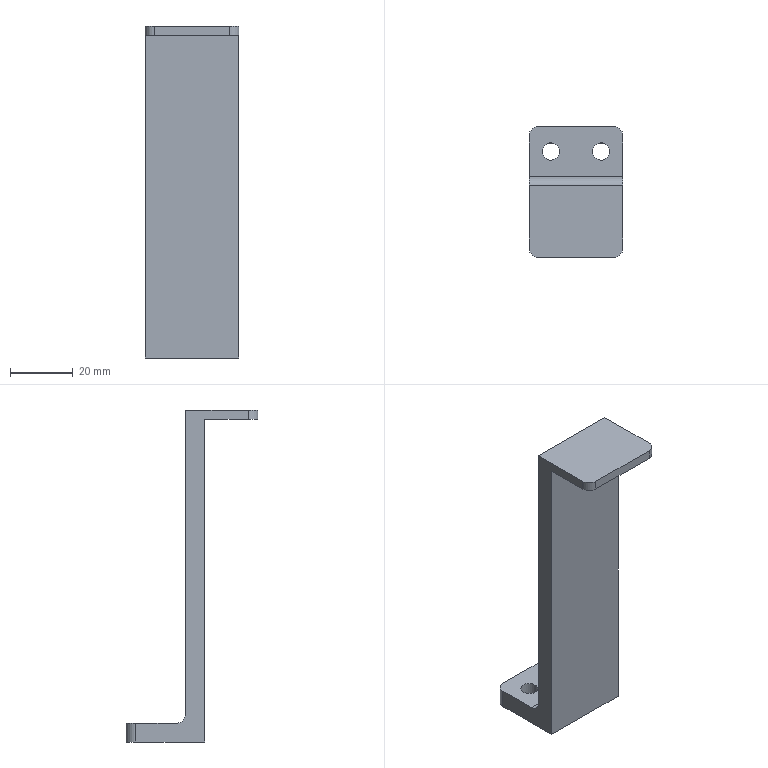Part | SolidWorks | features BaseBody 1 | 1 solid | 19 faces | box 30 x 42 x 106 mm | volume 23768 mm3 | plane 10 | cylinder 9 | commonest cylinder face diameters 6 x5 5.5 x4
STEP:
#1=CARTESIAN_POINT('',(-178.7,76.,-2.));
#2=VERTEX_POINT('',#1);
#3=CARTESIAN_POINT('',(-173.2,76.,-2.));
#4=VERTEX_POINT('',#3);
#5=CARTESIAN_POINT('',(-175.95,76.,-2.));
#6=DIRECTION('',(0.,0.,1.));
#7=DIRECTION('',(1.,0.,0.));
#8=AXIS2_PLACEMENT_3D('',#5,#6,#7);
#9=CIRCLE('',#8,2.75);
#10=EDGE_CURVE('',#2,#4,#9,.T.);
#11=ORIENTED_EDGE('',*,*,#10,.F.);
#12=CARTESIAN_POINT('',(-178.7,76.,4.));
#13=VERTEX_POINT('',#12);
#14=CARTESIAN_POINT('',(-178.7,76.,4.));
#15=DIRECTION('',(0.,0.,1.));
#16=VECTOR('',#15,1000.);
#17=LINE('',#14,#16);
#18=EDGE_CURVE('',#2,#13,#17,.T.);
#19=ORIENTED_EDGE('',*,*,#18,.T.);
#20=CARTESIAN_POINT('',(-173.2,76.,4.));
#21=VERTEX_POINT('',#20);
#22=CARTESIAN_POINT('',(-175.95,76.,4.));
#23=DIRECTION('',(0.,0.,-1.));
#24=DIRECTION('',(1.,0.,0.));
#25=AXIS2_PLACEMENT_3D('',#22,#23,#24);
#26=CIRCLE('',#25,2.75);
#27=EDGE_CURVE('',#21,#13,#26,.T.);
#28=ORIENTED_EDGE('',*,*,#27,.F.);
#29=CARTESIAN_POINT('',(-173.2,76.,4.));
#30=DIRECTION('',(0.,0.,1.));
#31=VECTOR('',#30,1000.);
#32=LINE('',#29,#31);
#33=EDGE_CURVE('',#4,#21,#32,.T.);
#34=ORIENTED_EDGE('',*,*,#33,.F.);
#35=EDGE_LOOP('',(#11,#19,#28,#34));
#36=FACE_OUTER_BOUND('',#35,.T.);
#37=CARTESIAN_POINT('',(-175.95,76.,4.));
#38=DIRECTION('',(0.,0.,1.));
#39=DIRECTION('',(1.,0.,0.));
#40=AXIS2_PLACEMENT_3D('',#37,#38,#39);
#41=CYLINDRICAL_SURFACE('',#40,2.75);
#42=ADVANCED_FACE('',(#36),#41,.F.);
#43=CARTESIAN_POINT('',(-162.7,76.,-2.));
#44=VERTEX_POINT('',#43);
#45=CARTESIAN_POINT('',(-157.2,76.,-2.));
#46=VERTEX_POINT('',#45);
#47=CARTESIAN_POINT('',(-159.95,76.,-2.));
#48=DIRECTION('',(0.,0.,1.));
#49=DIRECTION('',(1.,0.,0.));
#50=AXIS2_PLACEMENT_3D('',#47,#48,#49);
#51=CIRCLE('',#50,2.75);
#52=EDGE_CURVE('',#44,#46,#51,.T.);
#53=ORIENTED_EDGE('',*,*,#52,.F.);
#54=CARTESIAN_POINT('',(-162.7,76.,4.));
#55=VERTEX_POINT('',#54);
#56=CARTESIAN_POINT('',(-162.7,76.,4.));
#57=DIRECTION('',(0.,0.,1.));
#58=VECTOR('',#57,1000.);
#59=LINE('',#56,#58);
#60=EDGE_CURVE('',#44,#55,#59,.T.);
#61=ORIENTED_EDGE('',*,*,#60,.T.);
#62=CARTESIAN_POINT('',(-157.2,76.,4.));
#63=VERTEX_POINT('',#62);
#64=CARTESIAN_POINT('',(-159.95,76.,4.));
#65=DIRECTION('',(0.,0.,-1.));
#66=DIRECTION('',(1.,0.,0.));
#67=AXIS2_PLACEMENT_3D('',#64,#65,#66);
#68=CIRCLE('',#67,2.75);
#69=EDGE_CURVE('',#63,#55,#68,.T.);
#70=ORIENTED_EDGE('',*,*,#69,.F.);
#71=CARTESIAN_POINT('',(-157.2,76.,4.));
#72=DIRECTION('',(0.,0.,1.));
#73=VECTOR('',#72,1000.);
#74=LINE('',#71,#73);
#75=EDGE_CURVE('',#46,#63,#74,.T.);
#76=ORIENTED_EDGE('',*,*,#75,.F.);
#77=EDGE_LOOP('',(#53,#61,#70,#76));
#78=FACE_OUTER_BOUND('',#77,.T.);
#79=CARTESIAN_POINT('',(-159.95,76.,4.));
#80=DIRECTION('',(0.,0.,1.));
#81=DIRECTION('',(1.,0.,0.));
#82=AXIS2_PLACEMENT_3D('',#79,#80,#81);
#83=CYLINDRICAL_SURFACE('',#82,2.75);
#84=ADVANCED_FACE('',(#78),#83,.F.);
#85=CARTESIAN_POINT('',(-155.95,42.,104.));
#86=VERTEX_POINT('',#85);
#87=CARTESIAN_POINT('',(-179.95,42.,104.));
#88=VERTEX_POINT('',#87);
#89=CARTESIAN_POINT('',(-182.95,42.,104.));
#90=DIRECTION('',(-1.,0.,0.));
#91=VECTOR('',#90,1000.);
#92=LINE('',#89,#91);
#93=EDGE_CURVE('',#86,#88,#92,.T.);
#94=ORIENTED_EDGE('',*,*,#93,.T.);
#95=CARTESIAN_POINT('',(-179.95,42.,101.));
#96=VERTEX_POINT('',#95);
#97=CARTESIAN_POINT('',(-179.95,42.,-92.413));
#98=DIRECTION('',(0.,0.,1.));
#99=VECTOR('',#98,1000.);
#100=LINE('',#97,#99);
#101=EDGE_CURVE('',#96,#88,#100,.T.);
#102=ORIENTED_EDGE('',*,*,#101,.F.);
#103=CARTESIAN_POINT('',(-155.95,42.,101.));
#104=VERTEX_POINT('',#103);
#105=CARTESIAN_POINT('',(-182.95,42.,101.));
#106=DIRECTION('',(-1.,0.,0.));
#107=VECTOR('',#106,1000.);
#108=LINE('',#105,#107);
#109=EDGE_CURVE('',#104,#96,#108,.T.);
#110=ORIENTED_EDGE('',*,*,#109,.F.);
#111=CARTESIAN_POINT('',(-155.95,42.,221.413));
#112=DIRECTION('',(0.,0.,-1.));
#113=VECTOR('',#112,1000.);
#114=LINE('',#111,#113);
#115=EDGE_CURVE('',#86,#104,#114,.T.);
#116=ORIENTED_EDGE('',*,*,#115,.F.);
#117=EDGE_LOOP('',(#94,#102,#110,#116));
#118=FACE_OUTER_BOUND('',#117,.T.);
#119=CARTESIAN_POINT('',(-182.95,42.,108.));
#120=DIRECTION('',(0.,-1.,0.));
#121=DIRECTION('',(0.,0.,-1.));
#122=AXIS2_PLACEMENT_3D('',#119,#120,#121);
#123=PLANE('',#122);
#124=ADVANCED_FACE('',(#118),#123,.T.);
#125=CARTESIAN_POINT('',(-182.95,45.,104.));
#126=VERTEX_POINT('',#125);
#127=CARTESIAN_POINT('',(-179.95,45.,104.));
#128=DIRECTION('',(0.,0.,-1.));
#129=DIRECTION('',(1.,0.,0.));
#130=AXIS2_PLACEMENT_3D('',#127,#128,#129);
#131=CIRCLE('',#130,3.);
#132=EDGE_CURVE('',#88,#126,#131,.T.);
#133=ORIENTED_EDGE('',*,*,#132,.T.);
#134=CARTESIAN_POINT('',(-182.95,45.,101.));
#135=VERTEX_POINT('',#134);
#136=CARTESIAN_POINT('',(-182.95,45.,17.));
#137=DIRECTION('',(0.,0.,-1.));
#138=VECTOR('',#137,1000.);
#139=LINE('',#136,#138);
#140=EDGE_CURVE('',#126,#135,#139,.T.);
#141=ORIENTED_EDGE('',*,*,#140,.T.);
#142=CARTESIAN_POINT('',(-179.95,45.,101.));
#143=DIRECTION('',(0.,0.,-1.));
#144=DIRECTION('',(1.,0.,0.));
#145=AXIS2_PLACEMENT_3D('',#142,#143,#144);
#146=CIRCLE('',#145,3.);
#147=EDGE_CURVE('',#96,#135,#146,.T.);
#148=ORIENTED_EDGE('',*,*,#147,.F.);
#149=ORIENTED_EDGE('',*,*,#101,.T.);
#150=EDGE_LOOP('',(#133,#141,#148,#149));
#151=FACE_OUTER_BOUND('',#150,.T.);
#152=CARTESIAN_POINT('',(-179.95,45.,-92.413));
#153=DIRECTION('',(0.,0.,1.));
#154=DIRECTION('',(1.,0.,0.));
#155=AXIS2_PLACEMENT_3D('',#152,#153,#154);
#156=CYLINDRICAL_SURFACE('',#155,3.);
#157=ADVANCED_FACE('',(#151),#156,.T.);
#158=CARTESIAN_POINT('',(-179.95,84.,-2.));
#159=VERTEX_POINT('',#158);
#160=CARTESIAN_POINT('',(-155.95,84.,-2.));
#161=VERTEX_POINT('',#160);
#162=CARTESIAN_POINT('',(-182.95,84.,-2.));
#163=DIRECTION('',(1.,0.,0.));
#164=VECTOR('',#163,1000.);
#165=LINE('',#162,#164);
#166=EDGE_CURVE('',#159,#161,#165,.T.);
#167=ORIENTED_EDGE('',*,*,#166,.F.);
#168=CARTESIAN_POINT('',(-179.95,84.,4.));
#169=VERTEX_POINT('',#168);
#170=CARTESIAN_POINT('',(-179.95,84.,198.413));
#171=DIRECTION('',(0.,0.,-1.));
#172=VECTOR('',#171,1000.);
#173=LINE('',#170,#172);
#174=EDGE_CURVE('',#169,#159,#173,.T.);
#175=ORIENTED_EDGE('',*,*,#174,.F.);
#176=CARTESIAN_POINT('',(-155.95,84.,4.));
#177=VERTEX_POINT('',#176);
#178=CARTESIAN_POINT('',(-182.95,84.,4.));
#179=DIRECTION('',(-1.,0.,0.));
#180=VECTOR('',#179,1000.);
#181=LINE('',#178,#180);
#182=EDGE_CURVE('',#177,#169,#181,.T.);
#183=ORIENTED_EDGE('',*,*,#182,.F.);
#184=CARTESIAN_POINT('',(-155.95,84.,-115.413));
#185=DIRECTION('',(0.,0.,1.));
#186=VECTOR('',#185,1000.);
#187=LINE('',#184,#186);
#188=EDGE_CURVE('',#161,#177,#187,.T.);
#189=ORIENTED_EDGE('',*,*,#188,.F.);
#190=EDGE_LOOP('',(#167,#175,#183,#189));
#191=FACE_OUTER_BOUND('',#190,.T.);
#192=CARTESIAN_POINT('',(-182.95,84.,-2.));
#193=DIRECTION('',(0.,1.,0.));
#194=DIRECTION('',(1.,0.,0.));
#195=AXIS2_PLACEMENT_3D('',#192,#193,#194);
#196=PLANE('',#195);
#197=ADVANCED_FACE('',(#191),#196,.T.);
#198=CARTESIAN_POINT('',(-182.95,81.,-2.));
#199=VERTEX_POINT('',#198);
#200=CARTESIAN_POINT('',(-182.95,81.,4.));
#201=VERTEX_POINT('',#200);
#202=CARTESIAN_POINT('',(-182.95,81.,17.));
#203=DIRECTION('',(0.,0.,1.));
#204=VECTOR('',#203,1000.);
#205=LINE('',#202,#204);
#206=EDGE_CURVE('',#199,#201,#205,.T.);
#207=ORIENTED_EDGE('',*,*,#206,.T.);
#208=CARTESIAN_POINT('',(-179.95,81.,4.));
#209=DIRECTION('',(0.,0.,1.));
#210=DIRECTION('',(-1.,0.,0.));
#211=AXIS2_PLACEMENT_3D('',#208,#209,#210);
#212=CIRCLE('',#211,3.);
#213=EDGE_CURVE('',#169,#201,#212,.T.);
#214=ORIENTED_EDGE('',*,*,#213,.F.);
#215=ORIENTED_EDGE('',*,*,#174,.T.);
#216=CARTESIAN_POINT('',(-179.95,81.,-2.));
#217=DIRECTION('',(0.,0.,-1.));
#218=DIRECTION('',(-1.,0.,0.));
#219=AXIS2_PLACEMENT_3D('',#216,#217,#218);
#220=CIRCLE('',#219,3.);
#221=EDGE_CURVE('',#199,#159,#220,.T.);
#222=ORIENTED_EDGE('',*,*,#221,.F.);
#223=EDGE_LOOP('',(#207,#214,#215,#222));
#224=FACE_OUTER_BOUND('',#223,.T.);
#225=CARTESIAN_POINT('',(-179.95,81.,198.413));
#226=DIRECTION('',(0.,0.,-1.));
#227=DIRECTION('',(-1.,0.,0.));
#228=AXIS2_PLACEMENT_3D('',#225,#226,#227);
#229=CYLINDRICAL_SURFACE('',#228,3.);
#230=ADVANCED_FACE('',(#224),#229,.T.);
#231=CARTESIAN_POINT('',(-182.95,68.,4.));
#232=VERTEX_POINT('',#231);
#233=CARTESIAN_POINT('',(-182.95,65.,7.));
#234=VERTEX_POINT('',#233);
#235=CARTESIAN_POINT('',(-182.95,68.,7.));
#236=DIRECTION('',(-1.,0.,0.));
#237=DIRECTION('',(0.,0.,-1.));
#238=AXIS2_PLACEMENT_3D('',#235,#236,#237);
#239=CIRCLE('',#238,3.);
#240=EDGE_CURVE('',#232,#234,#239,.T.);
#241=ORIENTED_EDGE('',*,*,#240,.T.);
#242=CARTESIAN_POINT('',(-152.95,65.,7.));
#243=VERTEX_POINT('',#242);
#244=CARTESIAN_POINT('',(-182.95,65.,7.));
#245=DIRECTION('',(-1.,0.,0.));
#246=VECTOR('',#245,1000.);
#247=LINE('',#244,#246);
#248=EDGE_CURVE('',#243,#234,#247,.T.);
#249=ORIENTED_EDGE('',*,*,#248,.F.);
#250=CARTESIAN_POINT('',(-152.95,68.,4.));
#251=VERTEX_POINT('',#250);
#252=CARTESIAN_POINT('',(-152.95,68.,7.));
#253=DIRECTION('',(-1.,0.,0.));
#254=DIRECTION('',(0.,0.,-1.));
#255=AXIS2_PLACEMENT_3D('',#252,#253,#254);
#256=CIRCLE('',#255,3.);
#257=EDGE_CURVE('',#251,#243,#256,.T.);
#258=ORIENTED_EDGE('',*,*,#257,.F.);
#259=CARTESIAN_POINT('',(-182.95,68.,4.));
#260=DIRECTION('',(1.,0.,0.));
#261=VECTOR('',#260,1000.);
#262=LINE('',#259,#261);
#263=EDGE_CURVE('',#232,#251,#262,.T.);
#264=ORIENTED_EDGE('',*,*,#263,.F.);
#265=EDGE_LOOP('',(#241,#249,#258,#264));
#266=FACE_OUTER_BOUND('',#265,.T.);
#267=CARTESIAN_POINT('',(-222.058,68.,7.));
#268=DIRECTION('',(1.,0.,0.));
#269=DIRECTION('',(0.,0.,-1.));
#270=AXIS2_PLACEMENT_3D('',#267,#268,#269);
#271=CYLINDRICAL_SURFACE('',#270,3.);
#272=ADVANCED_FACE('',(#266),#271,.F.);
#273=CARTESIAN_POINT('',(-182.95,65.,104.));
#274=VERTEX_POINT('',#273);
#275=CARTESIAN_POINT('',(-152.95,65.,104.));
#276=VERTEX_POINT('',#275);
#277=CARTESIAN_POINT('',(-182.95,65.,104.));
#278=DIRECTION('',(1.,0.,0.));
#279=VECTOR('',#278,1000.);
#280=LINE('',#277,#279);
#281=EDGE_CURVE('',#274,#276,#280,.T.);
#282=ORIENTED_EDGE('',*,*,#281,.T.);
#283=CARTESIAN_POINT('',(-152.95,65.,17.));
#284=DIRECTION('',(0.,0.,1.));
#285=VECTOR('',#284,1000.);
#286=LINE('',#283,#285);
#287=EDGE_CURVE('',#243,#276,#286,.T.);
#288=ORIENTED_EDGE('',*,*,#287,.F.);
#289=ORIENTED_EDGE('',*,*,#248,.T.);
#290=CARTESIAN_POINT('',(-182.95,65.,17.));
#291=DIRECTION('',(0.,0.,1.));
#292=VECTOR('',#291,1000.);
#293=LINE('',#290,#292);
#294=EDGE_CURVE('',#234,#274,#293,.T.);
#295=ORIENTED_EDGE('',*,*,#294,.T.);
#296=EDGE_LOOP('',(#282,#288,#289,#295));
#297=FACE_OUTER_BOUND('',#296,.T.);
#298=CARTESIAN_POINT('',(-182.95,65.,4.));
#299=DIRECTION('',(0.,1.,0.));
#300=DIRECTION('',(1.,0.,0.));
#301=AXIS2_PLACEMENT_3D('',#298,#299,#300);
#302=PLANE('',#301);
#303=ADVANCED_FACE('',(#297),#302,.T.);
#304=ORIENTED_EDGE('',*,*,#132,.F.);
#305=ORIENTED_EDGE('',*,*,#93,.F.);
#306=CARTESIAN_POINT('',(-152.95,45.,104.));
#307=VERTEX_POINT('',#306);
#308=CARTESIAN_POINT('',(-155.95,45.,104.));
#309=DIRECTION('',(0.,0.,-1.));
#310=DIRECTION('',(-1.,0.,0.));
#311=AXIS2_PLACEMENT_3D('',#308,#309,#310);
#312=CIRCLE('',#311,3.);
#313=EDGE_CURVE('',#307,#86,#312,.T.);
#314=ORIENTED_EDGE('',*,*,#313,.F.);
#315=CARTESIAN_POINT('',(-152.95,9.5,104.));
#316=DIRECTION('',(0.,-1.,0.));
#317=VECTOR('',#316,1000.);
#318=LINE('',#315,#317);
#319=EDGE_CURVE('',#276,#307,#318,.T.);
#320=ORIENTED_EDGE('',*,*,#319,.F.);
#321=ORIENTED_EDGE('',*,*,#281,.F.);
#322=CARTESIAN_POINT('',(-182.95,9.5,104.));
#323=DIRECTION('',(0.,-1.,0.));
#324=VECTOR('',#323,1000.);
#325=LINE('',#322,#324);
#326=EDGE_CURVE('',#274,#126,#325,.T.);
#327=ORIENTED_EDGE('',*,*,#326,.T.);
#328=EDGE_LOOP('',(#304,#305,#314,#320,#321,#327));
#329=FACE_OUTER_BOUND('',#328,.T.);
#330=CARTESIAN_POINT('',(-182.95,84.,104.));
#331=DIRECTION('',(0.,0.,-1.));
#332=DIRECTION('',(0.,-1.,0.));
#333=AXIS2_PLACEMENT_3D('',#330,#331,#332);
#334=PLANE('',#333);
#335=ADVANCED_FACE('',(#329),#334,.F.);
#336=ORIENTED_EDGE('',*,*,#313,.T.);
#337=ORIENTED_EDGE('',*,*,#115,.T.);
#338=CARTESIAN_POINT('',(-152.95,45.,101.));
#339=VERTEX_POINT('',#338);
#340=CARTESIAN_POINT('',(-155.95,45.,101.));
#341=DIRECTION('',(0.,0.,-1.));
#342=DIRECTION('',(-1.,0.,0.));
#343=AXIS2_PLACEMENT_3D('',#340,#341,#342);
#344=CIRCLE('',#343,3.);
#345=EDGE_CURVE('',#339,#104,#344,.T.);
#346=ORIENTED_EDGE('',*,*,#345,.F.);
#347=CARTESIAN_POINT('',(-152.95,45.,17.));
#348=DIRECTION('',(0.,0.,-1.));
#349=VECTOR('',#348,1000.);
#350=LINE('',#347,#349);
#351=EDGE_CURVE('',#307,#339,#350,.T.);
#352=ORIENTED_EDGE('',*,*,#351,.F.);
#353=EDGE_LOOP('',(#336,#337,#346,#352));
#354=FACE_OUTER_BOUND('',#353,.T.);
#355=CARTESIAN_POINT('',(-155.95,45.,221.413));
#356=DIRECTION('',(0.,0.,-1.));
#357=DIRECTION('',(-1.,0.,0.));
#358=AXIS2_PLACEMENT_3D('',#355,#356,#357);
#359=CYLINDRICAL_SURFACE('',#358,3.);
#360=ADVANCED_FACE('',(#354),#359,.T.);
#361=CARTESIAN_POINT('',(-152.95,81.,-2.));
#362=VERTEX_POINT('',#361);
#363=CARTESIAN_POINT('',(-152.95,81.,4.));
#364=VERTEX_POINT('',#363);
#365=CARTESIAN_POINT('',(-152.95,81.,17.));
#366=DIRECTION('',(0.,0.,1.));
#367=VECTOR('',#366,1000.);
#368=LINE('',#365,#367);
#369=EDGE_CURVE('',#362,#364,#368,.T.);
#370=ORIENTED_EDGE('',*,*,#369,.F.);
#371=CARTESIAN_POINT('',(-155.95,81.,-2.));
#372=DIRECTION('',(0.,0.,-1.));
#373=DIRECTION('',(1.,0.,0.));
#374=AXIS2_PLACEMENT_3D('',#371,#372,#373);
#375=CIRCLE('',#374,3.);
#376=EDGE_CURVE('',#161,#362,#375,.T.);
#377=ORIENTED_EDGE('',*,*,#376,.F.);
#378=ORIENTED_EDGE('',*,*,#188,.T.);
#379=CARTESIAN_POINT('',(-155.95,81.,4.));
#380=DIRECTION('',(0.,0.,1.));
#381=DIRECTION('',(1.,0.,0.));
#382=AXIS2_PLACEMENT_3D('',#379,#380,#381);
#383=CIRCLE('',#382,3.);
#384=EDGE_CURVE('',#364,#177,#383,.T.);
#385=ORIENTED_EDGE('',*,*,#384,.F.);
#386=EDGE_LOOP('',(#370,#377,#378,#385));
#387=FACE_OUTER_BOUND('',#386,.T.);
#388=CARTESIAN_POINT('',(-155.95,81.,-115.413));
#389=DIRECTION('',(0.,0.,1.));
#390=DIRECTION('',(1.,0.,0.));
#391=AXIS2_PLACEMENT_3D('',#388,#389,#390);
#392=CYLINDRICAL_SURFACE('',#391,3.);
#393=ADVANCED_FACE('',(#387),#392,.T.);
#394=ORIENTED_EDGE('',*,*,#69,.T.);
#395=CARTESIAN_POINT('',(-159.95,76.,4.));
#396=DIRECTION('',(0.,0.,-1.));
#397=DIRECTION('',(1.,0.,0.));
#398=AXIS2_PLACEMENT_3D('',#395,#396,#397);
#399=CIRCLE('',#398,2.75);
#400=EDGE_CURVE('',#55,#63,#399,.T.);
#401=ORIENTED_EDGE('',*,*,#400,.T.);
#402=EDGE_LOOP('',(#394,#401));
#403=FACE_BOUND('',#402,.T.);
#404=ORIENTED_EDGE('',*,*,#27,.T.);
#405=CARTESIAN_POINT('',(-175.95,76.,4.));
#406=DIRECTION('',(0.,0.,-1.));
#407=DIRECTION('',(1.,0.,0.));
#408=AXIS2_PLACEMENT_3D('',#405,#406,#407);
#409=CIRCLE('',#408,2.75);
#410=EDGE_CURVE('',#13,#21,#409,.T.);
#411=ORIENTED_EDGE('',*,*,#410,.T.);
#412=EDGE_LOOP('',(#404,#411));
#413=FACE_BOUND('',#412,.T.);
#414=ORIENTED_EDGE('',*,*,#182,.T.);
#415=ORIENTED_EDGE('',*,*,#213,.T.);
#416=CARTESIAN_POINT('',(-182.95,9.5,4.));
#417=DIRECTION('',(0.,-1.,0.));
#418=VECTOR('',#417,1000.);
#419=LINE('',#416,#418);
#420=EDGE_CURVE('',#201,#232,#419,.T.);
#421=ORIENTED_EDGE('',*,*,#420,.T.);
#422=ORIENTED_EDGE('',*,*,#263,.T.);
#423=CARTESIAN_POINT('',(-152.95,9.5,4.));
#424=DIRECTION('',(0.,-1.,0.));
#425=VECTOR('',#424,1000.);
#426=LINE('',#423,#425);
#427=EDGE_CURVE('',#364,#251,#426,.T.);
#428=ORIENTED_EDGE('',*,*,#427,.F.);
#429=ORIENTED_EDGE('',*,*,#384,.T.);
#430=EDGE_LOOP('',(#414,#415,#421,#422,#428,#429));
#431=FACE_OUTER_BOUND('',#430,.T.);
#432=CARTESIAN_POINT('',(-182.95,84.,4.));
#433=DIRECTION('',(0.,0.,1.));
#434=DIRECTION('',(1.,0.,0.));
#435=AXIS2_PLACEMENT_3D('',#432,#433,#434);
#436=PLANE('',#435);
#437=ADVANCED_FACE('',(#403,#413,#431),#436,.T.);
#438=CARTESIAN_POINT('',(-182.95,59.,101.));
#439=VERTEX_POINT('',#438);
#440=CARTESIAN_POINT('',(-182.95,9.5,101.));
#441=DIRECTION('',(0.,1.,0.));
#442=VECTOR('',#441,1000.);
#443=LINE('',#440,#442);
#444=EDGE_CURVE('',#135,#439,#443,.T.);
#445=ORIENTED_EDGE('',*,*,#444,.T.);
#446=CARTESIAN_POINT('',(-152.95,59.,101.));
#447=VERTEX_POINT('',#446);
#448=CARTESIAN_POINT('',(-182.95,59.,101.));
#449=DIRECTION('',(-1.,0.,0.));
#450=VECTOR('',#449,1000.);
#451=LINE('',#448,#450);
#452=EDGE_CURVE('',#447,#439,#451,.T.);
#453=ORIENTED_EDGE('',*,*,#452,.F.);
#454=CARTESIAN_POINT('',(-152.95,9.5,101.));
#455=DIRECTION('',(0.,1.,0.));
#456=VECTOR('',#455,1000.);
#457=LINE('',#454,#456);
#458=EDGE_CURVE('',#339,#447,#457,.T.);
#459=ORIENTED_EDGE('',*,*,#458,.F.);
#460=ORIENTED_EDGE('',*,*,#345,.T.);
#461=ORIENTED_EDGE('',*,*,#109,.T.);
#462=ORIENTED_EDGE('',*,*,#147,.T.);
#463=EDGE_LOOP('',(#445,#453,#459,#460,#461,#462));
#464=FACE_OUTER_BOUND('',#463,.T.);
#465=CARTESIAN_POINT('',(-182.95,47.,101.));
#466=DIRECTION('',(0.,0.,-1.));
#467=DIRECTION('',(0.,-1.,0.));
#468=AXIS2_PLACEMENT_3D('',#465,#466,#467);
#469=PLANE('',#468);
#470=ADVANCED_FACE('',(#464),#469,.T.);
#471=ORIENTED_EDGE('',*,*,#294,.F.);
#472=ORIENTED_EDGE('',*,*,#240,.F.);
#473=ORIENTED_EDGE('',*,*,#420,.F.);
#474=ORIENTED_EDGE('',*,*,#206,.F.);
#475=CARTESIAN_POINT('',(-182.95,59.,-2.));
#476=VERTEX_POINT('',#475);
#477=CARTESIAN_POINT('',(-182.95,59.,-2.));
#478=DIRECTION('',(0.,1.,0.));
#479=VECTOR('',#478,1000.);
#480=LINE('',#477,#479);
#481=EDGE_CURVE('',#476,#199,#480,.T.);
#482=ORIENTED_EDGE('',*,*,#481,.F.);
#483=CARTESIAN_POINT('',(-182.95,59.,79.));
#484=DIRECTION('',(0.,0.,-1.));
#485=VECTOR('',#484,1000.);
#486=LINE('',#483,#485);
#487=EDGE_CURVE('',#439,#476,#486,.T.);
#488=ORIENTED_EDGE('',*,*,#487,.F.);
#489=ORIENTED_EDGE('',*,*,#444,.F.);
#490=ORIENTED_EDGE('',*,*,#140,.F.);
#491=ORIENTED_EDGE('',*,*,#326,.F.);
#492=EDGE_LOOP('',(#471,#472,#473,#474,#482,#488,#489,#490,#491));
#493=FACE_OUTER_BOUND('',#492,.T.);
#494=CARTESIAN_POINT('',(-182.95,9.5,17.));
#495=DIRECTION('',(1.,0.,0.));
#496=DIRECTION('',(0.,1.,0.));
#497=AXIS2_PLACEMENT_3D('',#494,#495,#496);
#498=PLANE('',#497);
#499=ADVANCED_FACE('',(#493),#498,.F.);
#500=CARTESIAN_POINT('',(-159.95,76.,-2.));
#501=DIRECTION('',(0.,0.,1.));
#502=DIRECTION('',(1.,0.,0.));
#503=AXIS2_PLACEMENT_3D('',#500,#501,#502);
#504=CIRCLE('',#503,2.75);
#505=EDGE_CURVE('',#46,#44,#504,.T.);
#506=ORIENTED_EDGE('',*,*,#505,.T.);
#507=ORIENTED_EDGE('',*,*,#52,.T.);
#508=EDGE_LOOP('',(#506,#507));
#509=FACE_BOUND('',#508,.T.);
#510=CARTESIAN_POINT('',(-175.95,76.,-2.));
#511=DIRECTION('',(0.,0.,1.));
#512=DIRECTION('',(1.,0.,0.));
#513=AXIS2_PLACEMENT_3D('',#510,#511,#512);
#514=CIRCLE('',#513,2.75);
#515=EDGE_CURVE('',#4,#2,#514,.T.);
#516=ORIENTED_EDGE('',*,*,#515,.T.);
#517=ORIENTED_EDGE('',*,*,#10,.T.);
#518=EDGE_LOOP('',(#516,#517));
#519=FACE_BOUND('',#518,.T.);
#520=ORIENTED_EDGE('',*,*,#481,.T.);
#521=ORIENTED_EDGE('',*,*,#221,.T.);
#522=ORIENTED_EDGE('',*,*,#166,.T.);
#523=ORIENTED_EDGE('',*,*,#376,.T.);
#524=CARTESIAN_POINT('',(-152.95,59.,-2.));
#525=VERTEX_POINT('',#524);
#526=CARTESIAN_POINT('',(-152.95,9.5,-2.));
#527=DIRECTION('',(0.,1.,0.));
#528=VECTOR('',#527,1000.);
#529=LINE('',#526,#528);
#530=EDGE_CURVE('',#525,#362,#529,.T.);
#531=ORIENTED_EDGE('',*,*,#530,.F.);
#532=CARTESIAN_POINT('',(-182.95,59.,-2.));
#533=DIRECTION('',(1.,0.,0.));
#534=VECTOR('',#533,1000.);
#535=LINE('',#532,#534);
#536=EDGE_CURVE('',#476,#525,#535,.T.);
#537=ORIENTED_EDGE('',*,*,#536,.F.);
#538=EDGE_LOOP('',(#520,#521,#522,#523,#531,#537));
#539=FACE_OUTER_BOUND('',#538,.T.);
#540=CARTESIAN_POINT('',(-182.95,59.,-2.));
#541=DIRECTION('',(0.,0.,-1.));
#542=DIRECTION('',(0.,-1.,0.));
#543=AXIS2_PLACEMENT_3D('',#540,#541,#542);
#544=PLANE('',#543);
#545=ADVANCED_FACE('',(#509,#519,#539),#544,.T.);
#546=ORIENTED_EDGE('',*,*,#369,.T.);
#547=ORIENTED_EDGE('',*,*,#427,.T.);
#548=ORIENTED_EDGE('',*,*,#257,.T.);
#549=ORIENTED_EDGE('',*,*,#287,.T.);
#550=ORIENTED_EDGE('',*,*,#319,.T.);
#551=ORIENTED_EDGE('',*,*,#351,.T.);
#552=ORIENTED_EDGE('',*,*,#458,.T.);
#553=CARTESIAN_POINT('',(-152.95,59.,79.));
#554=DIRECTION('',(0.,0.,1.));
#555=VECTOR('',#554,1000.);
#556=LINE('',#553,#555);
#557=EDGE_CURVE('',#525,#447,#556,.T.);
#558=ORIENTED_EDGE('',*,*,#557,.F.);
#559=ORIENTED_EDGE('',*,*,#530,.T.);
#560=EDGE_LOOP('',(#546,#547,#548,#549,#550,#551,#552,#558,#559));
#561=FACE_OUTER_BOUND('',#560,.T.);
#562=CARTESIAN_POINT('',(-152.95,9.5,17.));
#563=DIRECTION('',(1.,0.,0.));
#564=DIRECTION('',(0.,1.,0.));
#565=AXIS2_PLACEMENT_3D('',#562,#563,#564);
#566=PLANE('',#565);
#567=ADVANCED_FACE('',(#561),#566,.T.);
#568=ORIENTED_EDGE('',*,*,#536,.T.);
#569=ORIENTED_EDGE('',*,*,#557,.T.);
#570=ORIENTED_EDGE('',*,*,#452,.T.);
#571=ORIENTED_EDGE('',*,*,#487,.T.);
#572=EDGE_LOOP('',(#568,#569,#570,#571));
#573=FACE_OUTER_BOUND('',#572,.T.);
#574=CARTESIAN_POINT('',(-182.95,59.,79.));
#575=DIRECTION('',(0.,-1.,0.));
#576=DIRECTION('',(0.,0.,-1.));
#577=AXIS2_PLACEMENT_3D('',#574,#575,#576);
#578=PLANE('',#577);
#579=ADVANCED_FACE('',(#573),#578,.T.);
#580=ORIENTED_EDGE('',*,*,#60,.F.);
#581=ORIENTED_EDGE('',*,*,#505,.F.);
#582=ORIENTED_EDGE('',*,*,#75,.T.);
#583=ORIENTED_EDGE('',*,*,#400,.F.);
#584=EDGE_LOOP('',(#580,#581,#582,#583));
#585=FACE_OUTER_BOUND('',#584,.T.);
#586=CARTESIAN_POINT('',(-159.95,76.,4.));
#587=DIRECTION('',(0.,0.,1.));
#588=DIRECTION('',(1.,0.,0.));
#589=AXIS2_PLACEMENT_3D('',#586,#587,#588);
#590=CYLINDRICAL_SURFACE('',#589,2.75);
#591=ADVANCED_FACE('',(#585),#590,.F.);
#592=ORIENTED_EDGE('',*,*,#18,.F.);
#593=ORIENTED_EDGE('',*,*,#515,.F.);
#594=ORIENTED_EDGE('',*,*,#33,.T.);
#595=ORIENTED_EDGE('',*,*,#410,.F.);
#596=EDGE_LOOP('',(#592,#593,#594,#595));
#597=FACE_OUTER_BOUND('',#596,.T.);
#598=CARTESIAN_POINT('',(-175.95,76.,4.));
#599=DIRECTION('',(0.,0.,1.));
#600=DIRECTION('',(1.,0.,0.));
#601=AXIS2_PLACEMENT_3D('',#598,#599,#600);
#602=CYLINDRICAL_SURFACE('',#601,2.75);
#603=ADVANCED_FACE('',(#597),#602,.F.);
#604=CLOSED_SHELL('',(#42,#84,#124,#157,#197,#230,#272,#303,#335,#360,#393,#437,#470,#499,#545,#567,#579,#591,#603));
#605=MANIFOLD_SOLID_BREP('',#604);
#606=CARTESIAN_POINT('',(0.,0.,0.));
#607=DIRECTION('',(0.,0.,1.));
#608=DIRECTION('',(1.,0.,0.));
#609=AXIS2_PLACEMENT_3D('',#606,#607,#608);
#610=(LENGTH_UNIT()NAMED_UNIT(*)SI_UNIT(.MILLI.,.METRE.));
#611=UNCERTAINTY_MEASURE_WITH_UNIT(LENGTH_MEASURE(0.00001),#610,'','');
#612=(NAMED_UNIT(*)PLANE_ANGLE_UNIT()SI_UNIT($,.RADIAN.));
#613=(NAMED_UNIT(*)SI_UNIT($,.STERADIAN.)SOLID_ANGLE_UNIT());
#614=(GEOMETRIC_REPRESENTATION_CONTEXT(3)GLOBAL_UNCERTAINTY_ASSIGNED_CONTEXT((#611))GLOBAL_UNIT_ASSIGNED_CONTEXT((#610,#612,#613))REPRESENTATION_CONTEXT('',''));
#615=ADVANCED_BREP_SHAPE_REPRESENTATION('',(#605,#609),#614);